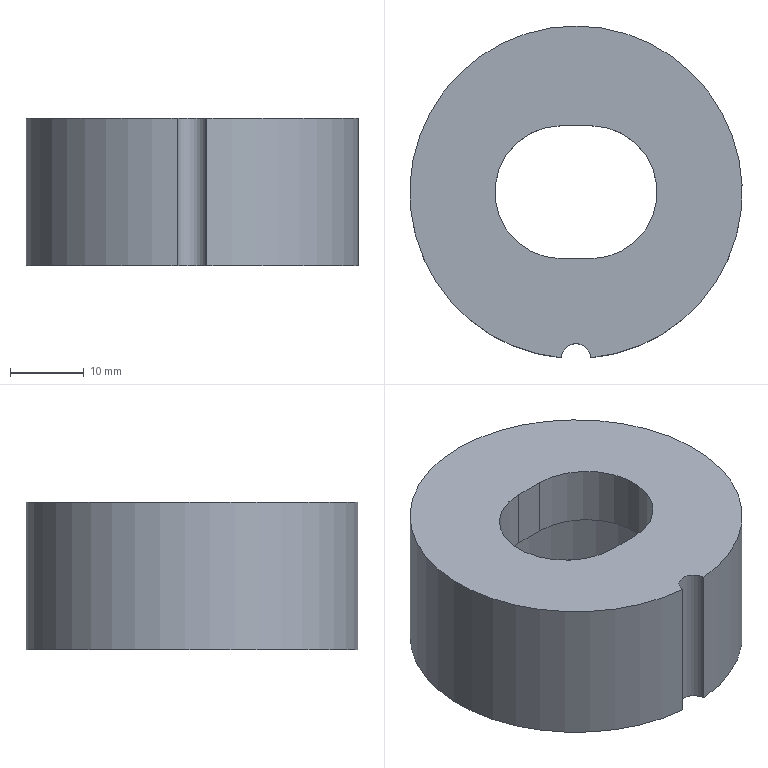Part | NX | features solid 2 | 1 solid | 10 faces | box 45 x 44.911 x 20 mm | volume 16859 mm3 | cylinder 5 | plane 5 | commonest cylinder face diameters 18 x2 4 x1 36 x1 45 x1
STEP:
#1=CARTESIAN_POINT('',(-223.002,-22.406,-20.));
#2=VERTEX_POINT('',#1);
#3=CARTESIAN_POINT('',(-223.002,-22.406,0.));
#4=VERTEX_POINT('',#3);
#5=CARTESIAN_POINT('',(-223.002,-22.406,-10.));
#6=DIRECTION('',(0.,0.,1.));
#7=VECTOR('',#6,1000.);
#8=LINE('',#5,#7);
#9=EDGE_CURVE('',#2,#4,#8,.T.);
#10=ORIENTED_EDGE('',*,*,#9,.F.);
#11=CARTESIAN_POINT('',(-226.998,-22.406,-20.));
#12=VERTEX_POINT('',#11);
#13=CARTESIAN_POINT('',(-225.,0.005131,-20.));
#14=DIRECTION('',(0.,0.,1.));
#15=DIRECTION('',(0.,-1.,0.));
#16=AXIS2_PLACEMENT_3D('',#13,#14,#15);
#17=CIRCLE('',#16,22.5);
#18=EDGE_CURVE('',#2,#12,#17,.T.);
#19=ORIENTED_EDGE('',*,*,#18,.T.);
#20=CARTESIAN_POINT('',(-226.998,-22.406,0.));
#21=VERTEX_POINT('',#20);
#22=CARTESIAN_POINT('',(-226.998,-22.406,-10.));
#23=DIRECTION('',(0.,0.,1.));
#24=VECTOR('',#23,1000.);
#25=LINE('',#22,#24);
#26=EDGE_CURVE('',#21,#12,#25,.F.);
#27=ORIENTED_EDGE('',*,*,#26,.F.);
#28=CARTESIAN_POINT('',(-225.,0.005131,0.));
#29=DIRECTION('',(0.,0.,1.));
#30=DIRECTION('',(1.,0.,0.));
#31=AXIS2_PLACEMENT_3D('',#28,#29,#30);
#32=CIRCLE('',#31,22.5);
#33=EDGE_CURVE('',#4,#21,#32,.T.);
#34=ORIENTED_EDGE('',*,*,#33,.F.);
#35=EDGE_LOOP('',(#10,#19,#27,#34));
#36=FACE_BOUND('',#35,.T.);
#37=CARTESIAN_POINT('',(-225.,0.005131,-20.));
#38=DIRECTION('',(0.,0.,1.));
#39=DIRECTION('',(0.,-1.,0.));
#40=AXIS2_PLACEMENT_3D('',#37,#38,#39);
#41=CYLINDRICAL_SURFACE('',#40,22.5);
#42=ADVANCED_FACE('',(#36),#41,.T.);
#43=CARTESIAN_POINT('',(-225.,-17.995,-20.));
#44=VERTEX_POINT('',#43);
#45=CARTESIAN_POINT('',(-225.,0.005131,-20.));
#46=DIRECTION('',(0.,0.,1.));
#47=DIRECTION('',(0.,-1.,0.));
#48=AXIS2_PLACEMENT_3D('',#45,#46,#47);
#49=CIRCLE('',#48,18.);
#50=EDGE_CURVE('',#44,#44,#49,.T.);
#51=ORIENTED_EDGE('',*,*,#50,.T.);
#52=EDGE_LOOP('',(#51));
#53=FACE_BOUND('',#52,.T.);
#54=ORIENTED_EDGE('',*,*,#18,.F.);
#55=CARTESIAN_POINT('',(-225.,-22.495,-20.));
#56=DIRECTION('',(0.,0.,1.));
#57=DIRECTION('',(0.,-1.,0.));
#58=AXIS2_PLACEMENT_3D('',#55,#56,#57);
#59=CIRCLE('',#58,2.);
#60=EDGE_CURVE('',#2,#12,#59,.T.);
#61=ORIENTED_EDGE('',*,*,#60,.T.);
#62=EDGE_LOOP('',(#54,#61));
#63=FACE_BOUND('',#62,.T.);
#64=CARTESIAN_POINT('',(-225.,0.005131,-20.));
#65=DIRECTION('',(0.,0.,1.));
#66=DIRECTION('',(0.,-1.,0.));
#67=AXIS2_PLACEMENT_3D('',#64,#65,#66);
#68=PLANE('',#67);
#69=ADVANCED_FACE('',(#53,#63),#68,.F.);
#70=CARTESIAN_POINT('',(-223.,9.005,0.));
#71=VERTEX_POINT('',#70);
#72=CARTESIAN_POINT('',(-227.,9.005,0.));
#73=VERTEX_POINT('',#72);
#74=CARTESIAN_POINT('',(-225.,9.005,0.));
#75=DIRECTION('',(-1.,0.,0.));
#76=VECTOR('',#75,1000.);
#77=LINE('',#74,#76);
#78=EDGE_CURVE('',#71,#73,#77,.T.);
#79=ORIENTED_EDGE('',*,*,#78,.F.);
#80=CARTESIAN_POINT('',(-223.,-8.995,0.));
#81=VERTEX_POINT('',#80);
#82=CARTESIAN_POINT('',(-223.,0.005131,0.));
#83=DIRECTION('',(0.,0.,1.));
#84=DIRECTION('',(1.,0.,0.));
#85=AXIS2_PLACEMENT_3D('',#82,#83,#84);
#86=CIRCLE('',#85,9.);
#87=EDGE_CURVE('',#81,#71,#86,.T.);
#88=ORIENTED_EDGE('',*,*,#87,.F.);
#89=CARTESIAN_POINT('',(-227.,-8.995,0.));
#90=VERTEX_POINT('',#89);
#91=CARTESIAN_POINT('',(-225.,-8.995,0.));
#92=DIRECTION('',(-1.,0.,0.));
#93=VECTOR('',#92,1000.);
#94=LINE('',#91,#93);
#95=EDGE_CURVE('',#81,#90,#94,.T.);
#96=ORIENTED_EDGE('',*,*,#95,.T.);
#97=CARTESIAN_POINT('',(-227.,0.005131,0.));
#98=DIRECTION('',(0.,0.,1.));
#99=DIRECTION('',(1.,0.,0.));
#100=AXIS2_PLACEMENT_3D('',#97,#98,#99);
#101=CIRCLE('',#100,9.);
#102=EDGE_CURVE('',#73,#90,#101,.T.);
#103=ORIENTED_EDGE('',*,*,#102,.F.);
#104=EDGE_LOOP('',(#79,#88,#96,#103));
#105=FACE_BOUND('',#104,.T.);
#106=CARTESIAN_POINT('',(-225.,-22.495,0.));
#107=DIRECTION('',(0.,0.,1.));
#108=DIRECTION('',(1.,0.,0.));
#109=AXIS2_PLACEMENT_3D('',#106,#107,#108);
#110=CIRCLE('',#109,2.);
#111=EDGE_CURVE('',#4,#21,#110,.T.);
#112=ORIENTED_EDGE('',*,*,#111,.F.);
#113=ORIENTED_EDGE('',*,*,#33,.T.);
#114=EDGE_LOOP('',(#112,#113));
#115=FACE_BOUND('',#114,.T.);
#116=CARTESIAN_POINT('',(-225.,0.005131,0.));
#117=DIRECTION('',(0.,0.,1.));
#118=DIRECTION('',(0.,-1.,0.));
#119=AXIS2_PLACEMENT_3D('',#116,#117,#118);
#120=PLANE('',#119);
#121=ADVANCED_FACE('',(#105,#115),#120,.T.);
#122=ORIENTED_EDGE('',*,*,#50,.F.);
#123=EDGE_LOOP('',(#122));
#124=FACE_BOUND('',#123,.T.);
#125=CARTESIAN_POINT('',(-225.,-17.995,-8.));
#126=VERTEX_POINT('',#125);
#127=CARTESIAN_POINT('',(-225.,0.005131,-8.));
#128=DIRECTION('',(0.,0.,1.));
#129=DIRECTION('',(0.,-1.,0.));
#130=AXIS2_PLACEMENT_3D('',#127,#128,#129);
#131=CIRCLE('',#130,18.);
#132=EDGE_CURVE('',#126,#126,#131,.T.);
#133=ORIENTED_EDGE('',*,*,#132,.T.);
#134=EDGE_LOOP('',(#133));
#135=FACE_BOUND('',#134,.T.);
#136=CARTESIAN_POINT('',(-225.,0.005131,-20.));
#137=DIRECTION('',(0.,0.,1.));
#138=DIRECTION('',(0.,-1.,0.));
#139=AXIS2_PLACEMENT_3D('',#136,#137,#138);
#140=CYLINDRICAL_SURFACE('',#139,18.);
#141=ADVANCED_FACE('',(#124,#135),#140,.F.);
#142=CARTESIAN_POINT('',(-223.,-8.995,-8.));
#143=VERTEX_POINT('',#142);
#144=CARTESIAN_POINT('',(-223.,9.005,-8.));
#145=VERTEX_POINT('',#144);
#146=CARTESIAN_POINT('',(-223.,0.005131,-8.));
#147=DIRECTION('',(0.,0.,1.));
#148=DIRECTION('',(0.,-1.,0.));
#149=AXIS2_PLACEMENT_3D('',#146,#147,#148);
#150=CIRCLE('',#149,9.);
#151=EDGE_CURVE('',#143,#145,#150,.T.);
#152=ORIENTED_EDGE('',*,*,#151,.T.);
#153=CARTESIAN_POINT('',(-227.,9.005,-8.));
#154=VERTEX_POINT('',#153);
#155=CARTESIAN_POINT('',(-225.,9.005,-8.));
#156=DIRECTION('',(-1.,0.,0.));
#157=VECTOR('',#156,1000.);
#158=LINE('',#155,#157);
#159=EDGE_CURVE('',#145,#154,#158,.T.);
#160=ORIENTED_EDGE('',*,*,#159,.T.);
#161=CARTESIAN_POINT('',(-227.,-8.995,-8.));
#162=VERTEX_POINT('',#161);
#163=CARTESIAN_POINT('',(-227.,0.005131,-8.));
#164=DIRECTION('',(0.,0.,1.));
#165=DIRECTION('',(0.,-1.,0.));
#166=AXIS2_PLACEMENT_3D('',#163,#164,#165);
#167=CIRCLE('',#166,9.);
#168=EDGE_CURVE('',#154,#162,#167,.T.);
#169=ORIENTED_EDGE('',*,*,#168,.T.);
#170=CARTESIAN_POINT('',(-225.,-8.995,-8.));
#171=DIRECTION('',(-1.,0.,0.));
#172=VECTOR('',#171,1000.);
#173=LINE('',#170,#172);
#174=EDGE_CURVE('',#143,#162,#173,.T.);
#175=ORIENTED_EDGE('',*,*,#174,.F.);
#176=EDGE_LOOP('',(#152,#160,#169,#175));
#177=FACE_BOUND('',#176,.T.);
#178=ORIENTED_EDGE('',*,*,#132,.F.);
#179=EDGE_LOOP('',(#178));
#180=FACE_BOUND('',#179,.T.);
#181=CARTESIAN_POINT('',(-225.,0.005131,-8.));
#182=DIRECTION('',(0.,0.,1.));
#183=DIRECTION('',(0.,-1.,0.));
#184=AXIS2_PLACEMENT_3D('',#181,#182,#183);
#185=PLANE('',#184);
#186=ADVANCED_FACE('',(#177,#180),#185,.F.);
#187=ORIENTED_EDGE('',*,*,#9,.T.);
#188=ORIENTED_EDGE('',*,*,#111,.T.);
#189=ORIENTED_EDGE('',*,*,#26,.T.);
#190=ORIENTED_EDGE('',*,*,#60,.F.);
#191=EDGE_LOOP('',(#187,#188,#189,#190));
#192=FACE_BOUND('',#191,.T.);
#193=CARTESIAN_POINT('',(-225.,-22.495,-20.));
#194=DIRECTION('',(0.,0.,1.));
#195=DIRECTION('',(0.,-1.,0.));
#196=AXIS2_PLACEMENT_3D('',#193,#194,#195);
#197=CYLINDRICAL_SURFACE('',#196,2.);
#198=ADVANCED_FACE('',(#192),#197,.F.);
#199=CARTESIAN_POINT('',(-223.,9.005,-20.));
#200=DIRECTION('',(0.,0.,1.));
#201=VECTOR('',#200,1000.);
#202=LINE('',#199,#201);
#203=EDGE_CURVE('',#145,#71,#202,.T.);
#204=ORIENTED_EDGE('',*,*,#203,.T.);
#205=ORIENTED_EDGE('',*,*,#78,.T.);
#206=CARTESIAN_POINT('',(-227.,9.005,-20.));
#207=DIRECTION('',(0.,0.,1.));
#208=VECTOR('',#207,1000.);
#209=LINE('',#206,#208);
#210=EDGE_CURVE('',#154,#73,#209,.T.);
#211=ORIENTED_EDGE('',*,*,#210,.F.);
#212=ORIENTED_EDGE('',*,*,#159,.F.);
#213=EDGE_LOOP('',(#204,#205,#211,#212));
#214=FACE_BOUND('',#213,.T.);
#215=CARTESIAN_POINT('',(-223.,9.005,-20.));
#216=DIRECTION('',(0.,1.,0.));
#217=DIRECTION('',(0.,0.,1.));
#218=AXIS2_PLACEMENT_3D('',#215,#216,#217);
#219=PLANE('',#218);
#220=ADVANCED_FACE('',(#214),#219,.F.);
#221=ORIENTED_EDGE('',*,*,#210,.T.);
#222=ORIENTED_EDGE('',*,*,#102,.T.);
#223=CARTESIAN_POINT('',(-227.,-8.995,-20.));
#224=DIRECTION('',(0.,0.,1.));
#225=VECTOR('',#224,1000.);
#226=LINE('',#223,#225);
#227=EDGE_CURVE('',#162,#90,#226,.T.);
#228=ORIENTED_EDGE('',*,*,#227,.F.);
#229=ORIENTED_EDGE('',*,*,#168,.F.);
#230=EDGE_LOOP('',(#221,#222,#228,#229));
#231=FACE_BOUND('',#230,.T.);
#232=CARTESIAN_POINT('',(-227.,0.005131,-20.));
#233=DIRECTION('',(0.,0.,1.));
#234=DIRECTION('',(0.,-1.,0.));
#235=AXIS2_PLACEMENT_3D('',#232,#233,#234);
#236=CYLINDRICAL_SURFACE('',#235,9.);
#237=ADVANCED_FACE('',(#231),#236,.F.);
#238=ORIENTED_EDGE('',*,*,#174,.T.);
#239=ORIENTED_EDGE('',*,*,#227,.T.);
#240=ORIENTED_EDGE('',*,*,#95,.F.);
#241=CARTESIAN_POINT('',(-223.,-8.995,-20.));
#242=DIRECTION('',(0.,0.,1.));
#243=VECTOR('',#242,1000.);
#244=LINE('',#241,#243);
#245=EDGE_CURVE('',#143,#81,#244,.T.);
#246=ORIENTED_EDGE('',*,*,#245,.F.);
#247=EDGE_LOOP('',(#238,#239,#240,#246));
#248=FACE_BOUND('',#247,.T.);
#249=CARTESIAN_POINT('',(-223.,-8.995,-20.));
#250=DIRECTION('',(0.,1.,0.));
#251=DIRECTION('',(0.,0.,1.));
#252=AXIS2_PLACEMENT_3D('',#249,#250,#251);
#253=PLANE('',#252);
#254=ADVANCED_FACE('',(#248),#253,.T.);
#255=ORIENTED_EDGE('',*,*,#245,.T.);
#256=ORIENTED_EDGE('',*,*,#87,.T.);
#257=ORIENTED_EDGE('',*,*,#203,.F.);
#258=ORIENTED_EDGE('',*,*,#151,.F.);
#259=EDGE_LOOP('',(#255,#256,#257,#258));
#260=FACE_BOUND('',#259,.T.);
#261=CARTESIAN_POINT('',(-223.,0.005131,-20.));
#262=DIRECTION('',(0.,0.,1.));
#263=DIRECTION('',(0.,-1.,0.));
#264=AXIS2_PLACEMENT_3D('',#261,#262,#263);
#265=CYLINDRICAL_SURFACE('',#264,9.);
#266=ADVANCED_FACE('',(#260),#265,.F.);
#267=CLOSED_SHELL('',(#42,#69,#121,#141,#186,#198,#220,#237,#254,#266));
#268=MANIFOLD_SOLID_BREP('',#267);
#269=(LENGTH_UNIT()NAMED_UNIT(*)SI_UNIT(.MILLI.,.METRE.));
#270=UNCERTAINTY_MEASURE_WITH_UNIT(LENGTH_MEASURE(0.00001),#269,'','');
#271=(NAMED_UNIT(*)PLANE_ANGLE_UNIT()SI_UNIT($,.RADIAN.));
#272=(NAMED_UNIT(*)SI_UNIT($,.STERADIAN.)SOLID_ANGLE_UNIT());
#273=(GEOMETRIC_REPRESENTATION_CONTEXT(3)GLOBAL_UNCERTAINTY_ASSIGNED_CONTEXT((#270))GLOBAL_UNIT_ASSIGNED_CONTEXT((#269,#271,#272))REPRESENTATION_CONTEXT('',''));
#274=ADVANCED_BREP_SHAPE_REPRESENTATION('',(#268),#273);